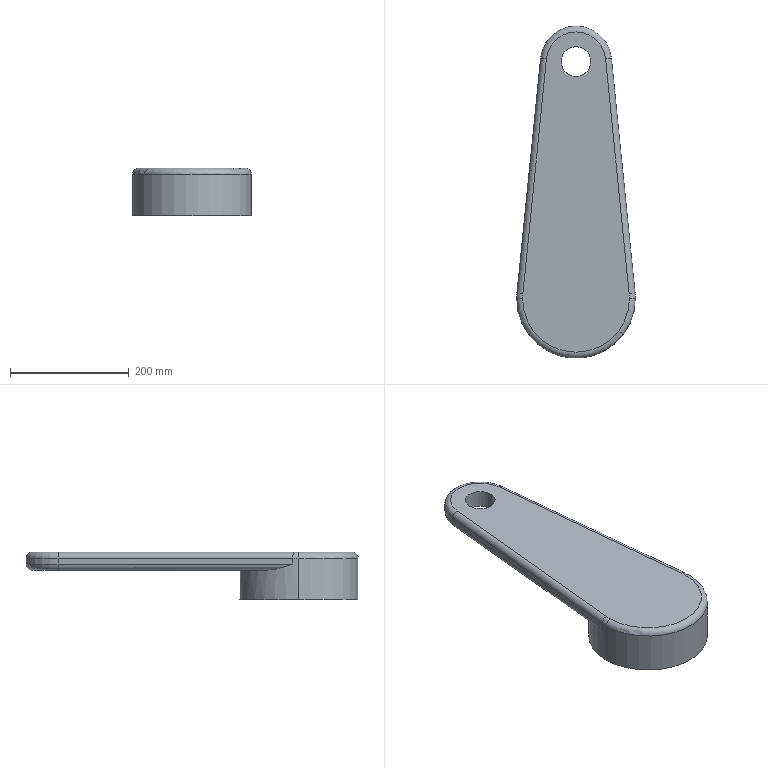Part | SolidWorks | features HoleWzd 2, Extrusion 1, Fillet 1, ICE 1 | 1 solid | 22 faces | box 200 x 560.023 x 80 mm | volume 3893750 mm3 | cylinder 11 | plane 6 | torus 5 | commonest cylinder face diameters 20 x4 50 x2 60 x2 200 x2 120.046 x1
STEP:
#1=CARTESIAN_POINT('',(90.,0.,30.));
#2=VERTEX_POINT('',#1);
#3=CARTESIAN_POINT('',(89.549,8.995,30.));
#4=VERTEX_POINT('',#3);
#5=CARTESIAN_POINT('',(0.,0.,30.));
#6=DIRECTION('',(0.,0.,1.));
#7=DIRECTION('',(-1.,0.,0.));
#8=AXIS2_PLACEMENT_3D('',#5,#6,#7);
#9=CIRCLE('',#8,90.);
#10=EDGE_CURVE('',#2,#4,#9,.T.);
#11=ORIENTED_EDGE('',*,*,#10,.F.);
#12=CARTESIAN_POINT('',(100.,0.,20.));
#13=VERTEX_POINT('',#12);
#14=CARTESIAN_POINT('',(90.,0.,20.));
#15=DIRECTION('',(0.,1.,0.));
#16=DIRECTION('',(-1.,0.,0.));
#17=AXIS2_PLACEMENT_3D('',#14,#15,#16);
#18=CIRCLE('',#17,10.);
#19=EDGE_CURVE('',#2,#13,#18,.T.);
#20=ORIENTED_EDGE('',*,*,#19,.T.);
#21=CARTESIAN_POINT('',(99.499,9.994,20.));
#22=VERTEX_POINT('',#21);
#23=CARTESIAN_POINT('',(0.,0.,20.));
#24=DIRECTION('',(0.,0.,-1.));
#25=DIRECTION('',(-1.,0.,0.));
#26=AXIS2_PLACEMENT_3D('',#23,#24,#25);
#27=CIRCLE('',#26,100.);
#28=EDGE_CURVE('',#22,#13,#27,.T.);
#29=ORIENTED_EDGE('',*,*,#28,.F.);
#30=CARTESIAN_POINT('',(89.549,8.995,20.));
#31=DIRECTION('',(0.09994,-0.995,0.));
#32=DIRECTION('',(0.995,0.09994,0.));
#33=AXIS2_PLACEMENT_3D('',#30,#31,#32);
#34=CIRCLE('',#33,10.);
#35=EDGE_CURVE('',#22,#4,#34,.T.);
#36=ORIENTED_EDGE('',*,*,#35,.T.);
#37=EDGE_LOOP('',(#11,#20,#29,#36));
#38=FACE_OUTER_BOUND('',#37,.T.);
#39=CARTESIAN_POINT('',(0.,0.,20.));
#40=DIRECTION('',(0.,0.,-1.));
#41=DIRECTION('',(-1.,0.,0.));
#42=AXIS2_PLACEMENT_3D('',#39,#40,#41);
#43=TOROIDAL_SURFACE('',#42,90.,10.);
#44=ADVANCED_FACE('',(#38),#43,.T.);
#45=ORIENTED_EDGE('',*,*,#19,.F.);
#46=CARTESIAN_POINT('',(-90.,0.,30.));
#47=VERTEX_POINT('',#46);
#48=CARTESIAN_POINT('',(0.,0.,30.));
#49=DIRECTION('',(0.,0.,1.));
#50=DIRECTION('',(-1.,0.,0.));
#51=AXIS2_PLACEMENT_3D('',#48,#49,#50);
#52=CIRCLE('',#51,90.);
#53=EDGE_CURVE('',#47,#2,#52,.T.);
#54=ORIENTED_EDGE('',*,*,#53,.F.);
#55=CARTESIAN_POINT('',(-100.,0.,20.));
#56=VERTEX_POINT('',#55);
#57=CARTESIAN_POINT('',(-90.,0.,20.));
#58=DIRECTION('',(0.,-1.,0.));
#59=DIRECTION('',(0.,0.,-1.));
#60=AXIS2_PLACEMENT_3D('',#57,#58,#59);
#61=CIRCLE('',#60,10.);
#62=EDGE_CURVE('',#47,#56,#61,.T.);
#63=ORIENTED_EDGE('',*,*,#62,.T.);
#64=CARTESIAN_POINT('',(0.,0.,20.));
#65=DIRECTION('',(0.,0.,-1.));
#66=DIRECTION('',(-1.,0.,0.));
#67=AXIS2_PLACEMENT_3D('',#64,#65,#66);
#68=CIRCLE('',#67,100.);
#69=EDGE_CURVE('',#13,#56,#68,.T.);
#70=ORIENTED_EDGE('',*,*,#69,.F.);
#71=EDGE_LOOP('',(#45,#54,#63,#70));
#72=FACE_OUTER_BOUND('',#71,.T.);
#73=CARTESIAN_POINT('',(0.,0.,20.));
#74=DIRECTION('',(0.,0.,-1.));
#75=DIRECTION('',(-1.,0.,0.));
#76=AXIS2_PLACEMENT_3D('',#73,#74,#75);
#77=TOROIDAL_SURFACE('',#76,90.,10.);
#78=ADVANCED_FACE('',(#72),#77,.T.);
#79=CARTESIAN_POINT('',(30.,0.,0.));
#80=VERTEX_POINT('',#79);
#81=CARTESIAN_POINT('',(-30.,0.,0.));
#82=VERTEX_POINT('',#81);
#83=CARTESIAN_POINT('',(0.,0.,0.));
#84=DIRECTION('',(0.,0.,-1.));
#85=DIRECTION('',(-1.,0.,0.));
#86=AXIS2_PLACEMENT_3D('',#83,#84,#85);
#87=CIRCLE('',#86,30.);
#88=EDGE_CURVE('',#80,#82,#87,.T.);
#89=ORIENTED_EDGE('',*,*,#88,.F.);
#90=CARTESIAN_POINT('',(30.,0.,-50.));
#91=VERTEX_POINT('',#90);
#92=CARTESIAN_POINT('',(30.,0.,-50.));
#93=DIRECTION('',(0.,0.,-1.));
#94=VECTOR('',#93,1000.);
#95=LINE('',#92,#94);
#96=EDGE_CURVE('',#80,#91,#95,.T.);
#97=ORIENTED_EDGE('',*,*,#96,.T.);
#98=CARTESIAN_POINT('',(-30.,0.,-50.));
#99=VERTEX_POINT('',#98);
#100=CARTESIAN_POINT('',(0.,0.,-50.));
#101=DIRECTION('',(0.,0.,-1.));
#102=DIRECTION('',(-1.,0.,0.));
#103=AXIS2_PLACEMENT_3D('',#100,#101,#102);
#104=CIRCLE('',#103,30.);
#105=EDGE_CURVE('',#91,#99,#104,.T.);
#106=ORIENTED_EDGE('',*,*,#105,.T.);
#107=CARTESIAN_POINT('',(-30.,0.,-50.));
#108=DIRECTION('',(0.,0.,-1.));
#109=VECTOR('',#108,1000.);
#110=LINE('',#107,#109);
#111=EDGE_CURVE('',#82,#99,#110,.T.);
#112=ORIENTED_EDGE('',*,*,#111,.F.);
#113=EDGE_LOOP('',(#89,#97,#106,#112));
#114=FACE_OUTER_BOUND('',#113,.T.);
#115=CARTESIAN_POINT('',(0.,0.,-50.));
#116=DIRECTION('',(0.,0.,-1.));
#117=DIRECTION('',(-1.,0.,0.));
#118=AXIS2_PLACEMENT_3D('',#115,#116,#117);
#119=CYLINDRICAL_SURFACE('',#118,30.);
#120=ADVANCED_FACE('',(#114),#119,.F.);
#121=CARTESIAN_POINT('',(25.,400.,30.));
#122=VERTEX_POINT('',#121);
#123=CARTESIAN_POINT('',(-25.,400.,30.));
#124=VERTEX_POINT('',#123);
#125=CARTESIAN_POINT('',(0.,400.,30.));
#126=DIRECTION('',(0.,0.,-1.));
#127=DIRECTION('',(-1.,0.,0.));
#128=AXIS2_PLACEMENT_3D('',#125,#126,#127);
#129=CIRCLE('',#128,25.);
#130=EDGE_CURVE('',#122,#124,#129,.T.);
#131=ORIENTED_EDGE('',*,*,#130,.F.);
#132=CARTESIAN_POINT('',(25.,400.,0.));
#133=VERTEX_POINT('',#132);
#134=CARTESIAN_POINT('',(25.,400.,0.));
#135=DIRECTION('',(0.,0.,-1.));
#136=VECTOR('',#135,1000.);
#137=LINE('',#134,#136);
#138=EDGE_CURVE('',#122,#133,#137,.T.);
#139=ORIENTED_EDGE('',*,*,#138,.T.);
#140=CARTESIAN_POINT('',(-25.,400.,0.));
#141=VERTEX_POINT('',#140);
#142=CARTESIAN_POINT('',(0.,400.,0.));
#143=DIRECTION('',(0.,0.,-1.));
#144=DIRECTION('',(-1.,0.,0.));
#145=AXIS2_PLACEMENT_3D('',#142,#143,#144);
#146=CIRCLE('',#145,25.);
#147=EDGE_CURVE('',#133,#141,#146,.T.);
#148=ORIENTED_EDGE('',*,*,#147,.T.);
#149=CARTESIAN_POINT('',(-25.,400.,0.));
#150=DIRECTION('',(0.,0.,-1.));
#151=VECTOR('',#150,1000.);
#152=LINE('',#149,#151);
#153=EDGE_CURVE('',#124,#141,#152,.T.);
#154=ORIENTED_EDGE('',*,*,#153,.F.);
#155=EDGE_LOOP('',(#131,#139,#148,#154));
#156=FACE_OUTER_BOUND('',#155,.T.);
#157=CARTESIAN_POINT('',(0.,400.,0.));
#158=DIRECTION('',(0.,0.,-1.));
#159=DIRECTION('',(-1.,0.,0.));
#160=AXIS2_PLACEMENT_3D('',#157,#158,#159);
#161=CYLINDRICAL_SURFACE('',#160,25.);
#162=ADVANCED_FACE('',(#156),#161,.F.);
#163=ORIENTED_EDGE('',*,*,#28,.T.);
#164=CARTESIAN_POINT('',(100.,0.,-50.));
#165=VERTEX_POINT('',#164);
#166=CARTESIAN_POINT('',(100.,0.,30.));
#167=DIRECTION('',(0.,0.,-1.));
#168=VECTOR('',#167,1000.);
#169=LINE('',#166,#168);
#170=EDGE_CURVE('',#13,#165,#169,.T.);
#171=ORIENTED_EDGE('',*,*,#170,.T.);
#172=CARTESIAN_POINT('',(-100.,0.,-50.));
#173=VERTEX_POINT('',#172);
#174=CARTESIAN_POINT('',(0.,0.,-50.));
#175=DIRECTION('',(0.,0.,-1.));
#176=DIRECTION('',(-1.,0.,0.));
#177=AXIS2_PLACEMENT_3D('',#174,#175,#176);
#178=CIRCLE('',#177,100.);
#179=EDGE_CURVE('',#173,#165,#178,.T.);
#180=ORIENTED_EDGE('',*,*,#179,.F.);
#181=CARTESIAN_POINT('',(-100.,0.,30.));
#182=DIRECTION('',(0.,0.,-1.));
#183=VECTOR('',#182,1000.);
#184=LINE('',#181,#183);
#185=EDGE_CURVE('',#56,#173,#184,.T.);
#186=ORIENTED_EDGE('',*,*,#185,.F.);
#187=CARTESIAN_POINT('',(-99.499,9.994,20.));
#188=VERTEX_POINT('',#187);
#189=CARTESIAN_POINT('',(0.,0.,20.));
#190=DIRECTION('',(0.,0.,-1.));
#191=DIRECTION('',(-1.,0.,0.));
#192=AXIS2_PLACEMENT_3D('',#189,#190,#191);
#193=CIRCLE('',#192,100.);
#194=EDGE_CURVE('',#56,#188,#193,.T.);
#195=ORIENTED_EDGE('',*,*,#194,.T.);
#196=CARTESIAN_POINT('',(-99.499,9.994,10.));
#197=VERTEX_POINT('',#196);
#198=CARTESIAN_POINT('',(-99.499,9.994,30.));
#199=DIRECTION('',(0.,0.,-1.));
#200=VECTOR('',#199,1000.);
#201=LINE('',#198,#200);
#202=EDGE_CURVE('',#188,#197,#201,.T.);
#203=ORIENTED_EDGE('',*,*,#202,.T.);
#204=CARTESIAN_POINT('',(-85.193,52.366,0.));
#205=VERTEX_POINT('',#204);
#206=CARTESIAN_POINT('',(-99.499,9.994,10.));
#207=CARTESIAN_POINT('',(-99.476,10.223,9.927));
#208=CARTESIAN_POINT('',(-99.452,10.454,9.854));
#209=CARTESIAN_POINT('',(-99.403,10.914,9.708));
#210=CARTESIAN_POINT('',(-99.326,11.603,9.489));
#211=CARTESIAN_POINT('',(-99.132,13.207,8.978));
#212=CARTESIAN_POINT('',(-98.936,14.576,8.544));
#213=CARTESIAN_POINT('',(-98.508,17.307,7.68));
#214=CARTESIAN_POINT('',(-98.173,19.118,7.111));
#215=CARTESIAN_POINT('',(-97.015,24.528,5.446));
#216=CARTESIAN_POINT('',(-96.043,28.102,4.387));
#217=CARTESIAN_POINT('',(-94.56,32.548,3.2));
#218=CARTESIAN_POINT('',(-94.249,33.436,2.97));
#219=CARTESIAN_POINT('',(-93.601,35.21,2.526));
#220=CARTESIAN_POINT('',(-93.263,36.097,2.312));
#221=CARTESIAN_POINT('',(-92.211,38.739,1.703));
#222=CARTESIAN_POINT('',(-91.46,40.482,1.339));
#223=CARTESIAN_POINT('',(-89.853,43.933,0.7212));
#224=CARTESIAN_POINT('',(-88.998,45.641,0.467));
#225=CARTESIAN_POINT('',(-87.179,49.026,0.1067));
#226=CARTESIAN_POINT('',(-86.215,50.702,0.));
#227=CARTESIAN_POINT('',(-85.193,52.366,0.));
#228=B_SPLINE_CURVE_WITH_KNOTS('',3,(#206,#207,#208,#209,#210,#211,#212,#213,#214,#215,#216,#217,#218,#219,#220,#221,#222,#223,#224,#225,#226,#227),.UNSPECIFIED.,.F.,.F.,(4,2,1,1,2,2,2,2,2,2,2,4),(-0.00006325,0.0006587,0.001381,0.002825,0.005713,0.01149,0.02304,0.02593,0.02882,0.03459,0.04037,0.04614),.UNSPECIFIED.);
#229=EDGE_CURVE('',#197,#205,#228,.T.);
#230=ORIENTED_EDGE('',*,*,#229,.T.);
#231=CARTESIAN_POINT('',(85.193,52.366,0.));
#232=VERTEX_POINT('',#231);
#233=CARTESIAN_POINT('',(0.,0.,0.));
#234=DIRECTION('',(0.,0.,-1.));
#235=DIRECTION('',(-1.,0.,0.));
#236=AXIS2_PLACEMENT_3D('',#233,#234,#235);
#237=CIRCLE('',#236,100.);
#238=EDGE_CURVE('',#205,#232,#237,.T.);
#239=ORIENTED_EDGE('',*,*,#238,.T.);
#240=CARTESIAN_POINT('',(99.499,9.994,10.));
#241=VERTEX_POINT('',#240);
#242=CARTESIAN_POINT('',(85.193,52.366,0.));
#243=CARTESIAN_POINT('',(86.215,50.702,0.));
#244=CARTESIAN_POINT('',(87.179,49.026,0.1067));
#245=CARTESIAN_POINT('',(88.998,45.641,0.4669));
#246=CARTESIAN_POINT('',(89.853,43.933,0.7212));
#247=CARTESIAN_POINT('',(91.46,40.482,1.339));
#248=CARTESIAN_POINT('',(92.211,38.739,1.703));
#249=CARTESIAN_POINT('',(93.263,36.097,2.312));
#250=CARTESIAN_POINT('',(93.601,35.21,2.526));
#251=CARTESIAN_POINT('',(94.249,33.436,2.97));
#252=CARTESIAN_POINT('',(94.56,32.548,3.2));
#253=CARTESIAN_POINT('',(96.043,28.102,4.387));
#254=CARTESIAN_POINT('',(97.015,24.528,5.446));
#255=CARTESIAN_POINT('',(98.173,19.118,7.111));
#256=CARTESIAN_POINT('',(98.508,17.307,7.68));
#257=CARTESIAN_POINT('',(98.936,14.576,8.544));
#258=CARTESIAN_POINT('',(99.066,13.663,8.833));
#259=CARTESIAN_POINT('',(99.243,12.29,9.27));
#260=CARTESIAN_POINT('',(99.326,11.603,9.489));
#261=CARTESIAN_POINT('',(99.403,10.914,9.708));
#262=CARTESIAN_POINT('',(99.452,10.454,9.854));
#263=CARTESIAN_POINT('',(99.476,10.223,9.927));
#264=CARTESIAN_POINT('',(99.499,9.994,10.));
#265=B_SPLINE_CURVE_WITH_KNOTS('',3,(#242,#243,#244,#245,#246,#247,#248,#249,#250,#251,#252,#253,#254,#255,#256,#257,#258,#259,#260,#261,#262,#263,#264),.UNSPECIFIED.,.F.,.F.,(4,2,2,2,2,2,2,2,2,1,2,4),(0.,0.005781,0.01156,0.01734,0.02023,0.02312,0.03469,0.04047,0.04336,0.0448,0.04553,0.04625),.UNSPECIFIED.);
#266=EDGE_CURVE('',#232,#241,#265,.T.);
#267=ORIENTED_EDGE('',*,*,#266,.T.);
#268=CARTESIAN_POINT('',(99.499,9.994,30.));
#269=DIRECTION('',(0.,0.,-1.));
#270=VECTOR('',#269,1000.);
#271=LINE('',#268,#270);
#272=EDGE_CURVE('',#22,#241,#271,.T.);
#273=ORIENTED_EDGE('',*,*,#272,.F.);
#274=EDGE_LOOP('',(#163,#171,#180,#186,#195,#203,#230,#239,#267,#273));
#275=FACE_OUTER_BOUND('',#274,.T.);
#276=CARTESIAN_POINT('',(0.,0.,30.));
#277=DIRECTION('',(0.,0.,-1.));
#278=DIRECTION('',(-1.,0.,0.));
#279=AXIS2_PLACEMENT_3D('',#276,#277,#278);
#280=CYLINDRICAL_SURFACE('',#279,100.);
#281=ADVANCED_FACE('',(#275),#280,.T.);
#282=CARTESIAN_POINT('',(-59.723,405.999,20.));
#283=VERTEX_POINT('',#282);
#284=CARTESIAN_POINT('',(-59.723,405.999,10.));
#285=VERTEX_POINT('',#284);
#286=CARTESIAN_POINT('',(-59.723,405.999,30.));
#287=DIRECTION('',(0.,0.,-1.));
#288=VECTOR('',#287,1000.);
#289=LINE('',#286,#288);
#290=EDGE_CURVE('',#283,#285,#289,.T.);
#291=ORIENTED_EDGE('',*,*,#290,.F.);
#292=CARTESIAN_POINT('',(59.723,405.999,20.));
#293=VERTEX_POINT('',#292);
#294=CARTESIAN_POINT('',(0.,400.,20.));
#295=DIRECTION('',(0.,0.,-1.));
#296=DIRECTION('',(-1.,0.,0.));
#297=AXIS2_PLACEMENT_3D('',#294,#295,#296);
#298=CIRCLE('',#297,60.023);
#299=EDGE_CURVE('',#283,#293,#298,.T.);
#300=ORIENTED_EDGE('',*,*,#299,.T.);
#301=CARTESIAN_POINT('',(59.723,405.999,10.));
#302=VERTEX_POINT('',#301);
#303=CARTESIAN_POINT('',(59.723,405.999,30.));
#304=DIRECTION('',(0.,0.,-1.));
#305=VECTOR('',#304,1000.);
#306=LINE('',#303,#305);
#307=EDGE_CURVE('',#293,#302,#306,.T.);
#308=ORIENTED_EDGE('',*,*,#307,.T.);
#309=CARTESIAN_POINT('',(0.,400.,10.));
#310=DIRECTION('',(0.,0.,1.));
#311=DIRECTION('',(-1.,0.,0.));
#312=AXIS2_PLACEMENT_3D('',#309,#310,#311);
#313=CIRCLE('',#312,60.023);
#314=EDGE_CURVE('',#302,#285,#313,.T.);
#315=ORIENTED_EDGE('',*,*,#314,.T.);
#316=EDGE_LOOP('',(#291,#300,#308,#315));
#317=FACE_OUTER_BOUND('',#316,.T.);
#318=CARTESIAN_POINT('',(0.,400.,30.));
#319=DIRECTION('',(0.,0.,-1.));
#320=DIRECTION('',(-1.,0.,0.));
#321=AXIS2_PLACEMENT_3D('',#318,#319,#320);
#322=CYLINDRICAL_SURFACE('',#321,60.023);
#323=ADVANCED_FACE('',(#317),#322,.T.);
#324=ORIENTED_EDGE('',*,*,#202,.F.);
#325=CARTESIAN_POINT('',(-59.723,405.999,20.));
#326=DIRECTION('',(0.09994,0.995,0.));
#327=VECTOR('',#326,1000.);
#328=LINE('',#325,#327);
#329=EDGE_CURVE('',#188,#283,#328,.T.);
#330=ORIENTED_EDGE('',*,*,#329,.T.);
#331=ORIENTED_EDGE('',*,*,#290,.T.);
#332=CARTESIAN_POINT('',(-99.499,9.994,10.));
#333=DIRECTION('',(-0.09994,-0.995,0.));
#334=VECTOR('',#333,1000.);
#335=LINE('',#332,#334);
#336=EDGE_CURVE('',#285,#197,#335,.T.);
#337=ORIENTED_EDGE('',*,*,#336,.T.);
#338=EDGE_LOOP('',(#324,#330,#331,#337));
#339=FACE_OUTER_BOUND('',#338,.T.);
#340=CARTESIAN_POINT('',(-99.499,9.994,30.));
#341=DIRECTION('',(-0.995,0.09994,0.));
#342=DIRECTION('',(-0.09994,-0.995,0.));
#343=AXIS2_PLACEMENT_3D('',#340,#341,#342);
#344=PLANE('',#343);
#345=ADVANCED_FACE('',(#339),#344,.T.);
#346=ORIENTED_EDGE('',*,*,#170,.F.);
#347=ORIENTED_EDGE('',*,*,#69,.T.);
#348=ORIENTED_EDGE('',*,*,#185,.T.);
#349=CARTESIAN_POINT('',(0.,0.,-50.));
#350=DIRECTION('',(0.,0.,-1.));
#351=DIRECTION('',(-1.,0.,0.));
#352=AXIS2_PLACEMENT_3D('',#349,#350,#351);
#353=CIRCLE('',#352,100.);
#354=EDGE_CURVE('',#165,#173,#353,.T.);
#355=ORIENTED_EDGE('',*,*,#354,.F.);
#356=EDGE_LOOP('',(#346,#347,#348,#355));
#357=FACE_OUTER_BOUND('',#356,.T.);
#358=CARTESIAN_POINT('',(0.,0.,30.));
#359=DIRECTION('',(0.,0.,-1.));
#360=DIRECTION('',(-1.,0.,0.));
#361=AXIS2_PLACEMENT_3D('',#358,#359,#360);
#362=CYLINDRICAL_SURFACE('',#361,100.);
#363=ADVANCED_FACE('',(#357),#362,.T.);
#364=ORIENTED_EDGE('',*,*,#307,.F.);
#365=CARTESIAN_POINT('',(99.499,9.994,20.));
#366=DIRECTION('',(0.09994,-0.995,0.));
#367=VECTOR('',#366,1000.);
#368=LINE('',#365,#367);
#369=EDGE_CURVE('',#293,#22,#368,.T.);
#370=ORIENTED_EDGE('',*,*,#369,.T.);
#371=ORIENTED_EDGE('',*,*,#272,.T.);
#372=CARTESIAN_POINT('',(59.723,405.999,10.));
#373=DIRECTION('',(-0.09994,0.995,0.));
#374=VECTOR('',#373,1000.);
#375=LINE('',#372,#374);
#376=EDGE_CURVE('',#241,#302,#375,.T.);
#377=ORIENTED_EDGE('',*,*,#376,.T.);
#378=EDGE_LOOP('',(#364,#370,#371,#377));
#379=FACE_OUTER_BOUND('',#378,.T.);
#380=CARTESIAN_POINT('',(59.723,405.999,30.));
#381=DIRECTION('',(0.995,0.09994,0.));
#382=DIRECTION('',(-0.09994,0.995,0.));
#383=AXIS2_PLACEMENT_3D('',#380,#381,#382);
#384=PLANE('',#383);
#385=ADVANCED_FACE('',(#379),#384,.T.);
#386=CARTESIAN_POINT('',(-49.773,404.999,30.));
#387=VERTEX_POINT('',#386);
#388=CARTESIAN_POINT('',(-89.549,8.995,30.));
#389=VERTEX_POINT('',#388);
#390=CARTESIAN_POINT('',(-89.549,8.995,30.));
#391=DIRECTION('',(-0.09994,-0.995,0.));
#392=VECTOR('',#391,1000.);
#393=LINE('',#390,#392);
#394=EDGE_CURVE('',#387,#389,#393,.T.);
#395=ORIENTED_EDGE('',*,*,#394,.T.);
#396=CARTESIAN_POINT('',(0.,0.,30.));
#397=DIRECTION('',(0.,0.,1.));
#398=DIRECTION('',(-1.,0.,0.));
#399=AXIS2_PLACEMENT_3D('',#396,#397,#398);
#400=CIRCLE('',#399,90.);
#401=EDGE_CURVE('',#389,#47,#400,.T.);
#402=ORIENTED_EDGE('',*,*,#401,.T.);
#403=ORIENTED_EDGE('',*,*,#53,.T.);
#404=ORIENTED_EDGE('',*,*,#10,.T.);
#405=CARTESIAN_POINT('',(49.773,404.999,30.));
#406=VERTEX_POINT('',#405);
#407=CARTESIAN_POINT('',(49.773,404.999,30.));
#408=DIRECTION('',(-0.09994,0.995,0.));
#409=VECTOR('',#408,1000.);
#410=LINE('',#407,#409);
#411=EDGE_CURVE('',#4,#406,#410,.T.);
#412=ORIENTED_EDGE('',*,*,#411,.T.);
#413=CARTESIAN_POINT('',(0.,400.,30.));
#414=DIRECTION('',(0.,0.,1.));
#415=DIRECTION('',(-1.,0.,0.));
#416=AXIS2_PLACEMENT_3D('',#413,#414,#415);
#417=CIRCLE('',#416,50.023);
#418=EDGE_CURVE('',#406,#387,#417,.T.);
#419=ORIENTED_EDGE('',*,*,#418,.T.);
#420=EDGE_LOOP('',(#395,#402,#403,#404,#412,#419));
#421=FACE_OUTER_BOUND('',#420,.T.);
#422=CARTESIAN_POINT('',(0.,400.,30.));
#423=DIRECTION('',(0.,0.,-1.));
#424=DIRECTION('',(-1.,0.,0.));
#425=AXIS2_PLACEMENT_3D('',#422,#423,#424);
#426=CIRCLE('',#425,25.);
#427=EDGE_CURVE('',#124,#122,#426,.T.);
#428=ORIENTED_EDGE('',*,*,#427,.T.);
#429=ORIENTED_EDGE('',*,*,#130,.T.);
#430=EDGE_LOOP('',(#428,#429));
#431=FACE_BOUND('',#430,.T.);
#432=CARTESIAN_POINT('',(0.,400.,30.));
#433=DIRECTION('',(0.,0.,-1.));
#434=DIRECTION('',(-1.,0.,0.));
#435=AXIS2_PLACEMENT_3D('',#432,#433,#434);
#436=PLANE('',#435);
#437=ADVANCED_FACE('',(#421,#431),#436,.F.);
#438=ORIENTED_EDGE('',*,*,#238,.F.);
#439=CARTESIAN_POINT('',(-49.773,404.999,0.));
#440=VERTEX_POINT('',#439);
#441=CARTESIAN_POINT('',(-49.773,404.999,0.));
#442=DIRECTION('',(0.09994,0.995,0.));
#443=VECTOR('',#442,1000.);
#444=LINE('',#441,#443);
#445=EDGE_CURVE('',#205,#440,#444,.T.);
#446=ORIENTED_EDGE('',*,*,#445,.T.);
#447=CARTESIAN_POINT('',(49.773,404.999,0.));
#448=VERTEX_POINT('',#447);
#449=CARTESIAN_POINT('',(0.,400.,0.));
#450=DIRECTION('',(0.,0.,-1.));
#451=DIRECTION('',(-1.,0.,0.));
#452=AXIS2_PLACEMENT_3D('',#449,#450,#451);
#453=CIRCLE('',#452,50.023);
#454=EDGE_CURVE('',#440,#448,#453,.T.);
#455=ORIENTED_EDGE('',*,*,#454,.T.);
#456=CARTESIAN_POINT('',(49.773,404.999,0.));
#457=DIRECTION('',(0.09994,-0.995,0.));
#458=VECTOR('',#457,1000.);
#459=LINE('',#456,#458);
#460=EDGE_CURVE('',#448,#232,#459,.T.);
#461=ORIENTED_EDGE('',*,*,#460,.T.);
#462=EDGE_LOOP('',(#438,#446,#455,#461));
#463=FACE_OUTER_BOUND('',#462,.T.);
#464=CARTESIAN_POINT('',(0.,400.,0.));
#465=DIRECTION('',(0.,0.,-1.));
#466=DIRECTION('',(-1.,0.,0.));
#467=AXIS2_PLACEMENT_3D('',#464,#465,#466);
#468=CIRCLE('',#467,25.);
#469=EDGE_CURVE('',#141,#133,#468,.T.);
#470=ORIENTED_EDGE('',*,*,#469,.F.);
#471=ORIENTED_EDGE('',*,*,#147,.F.);
#472=EDGE_LOOP('',(#470,#471));
#473=FACE_BOUND('',#472,.T.);
#474=CARTESIAN_POINT('',(0.,400.,0.));
#475=DIRECTION('',(0.,0.,-1.));
#476=DIRECTION('',(-1.,0.,0.));
#477=AXIS2_PLACEMENT_3D('',#474,#475,#476);
#478=PLANE('',#477);
#479=ADVANCED_FACE('',(#463,#473),#478,.T.);
#480=CARTESIAN_POINT('',(0.,0.,-50.));
#481=DIRECTION('',(0.,0.,-1.));
#482=DIRECTION('',(-1.,0.,0.));
#483=AXIS2_PLACEMENT_3D('',#480,#481,#482);
#484=CIRCLE('',#483,30.);
#485=EDGE_CURVE('',#99,#91,#484,.T.);
#486=ORIENTED_EDGE('',*,*,#485,.F.);
#487=ORIENTED_EDGE('',*,*,#105,.F.);
#488=EDGE_LOOP('',(#486,#487));
#489=FACE_BOUND('',#488,.T.);
#490=ORIENTED_EDGE('',*,*,#179,.T.);
#491=ORIENTED_EDGE('',*,*,#354,.T.);
#492=EDGE_LOOP('',(#490,#491));
#493=FACE_OUTER_BOUND('',#492,.T.);
#494=CARTESIAN_POINT('',(0.,0.,-50.));
#495=DIRECTION('',(0.,0.,-1.));
#496=DIRECTION('',(-1.,0.,0.));
#497=AXIS2_PLACEMENT_3D('',#494,#495,#496);
#498=PLANE('',#497);
#499=ADVANCED_FACE('',(#489,#493),#498,.T.);
#500=ORIENTED_EDGE('',*,*,#138,.F.);
#501=ORIENTED_EDGE('',*,*,#427,.F.);
#502=ORIENTED_EDGE('',*,*,#153,.T.);
#503=ORIENTED_EDGE('',*,*,#469,.T.);
#504=EDGE_LOOP('',(#500,#501,#502,#503));
#505=FACE_OUTER_BOUND('',#504,.T.);
#506=CARTESIAN_POINT('',(0.,400.,0.));
#507=DIRECTION('',(0.,0.,-1.));
#508=DIRECTION('',(-1.,0.,0.));
#509=AXIS2_PLACEMENT_3D('',#506,#507,#508);
#510=CYLINDRICAL_SURFACE('',#509,25.);
#511=ADVANCED_FACE('',(#505),#510,.F.);
#512=CARTESIAN_POINT('',(0.,0.,0.));
#513=DIRECTION('',(0.,0.,-1.));
#514=DIRECTION('',(-1.,0.,0.));
#515=AXIS2_PLACEMENT_3D('',#512,#513,#514);
#516=CIRCLE('',#515,30.);
#517=EDGE_CURVE('',#82,#80,#516,.T.);
#518=ORIENTED_EDGE('',*,*,#517,.T.);
#519=ORIENTED_EDGE('',*,*,#88,.T.);
#520=EDGE_LOOP('',(#518,#519));
#521=FACE_OUTER_BOUND('',#520,.T.);
#522=CARTESIAN_POINT('',(0.,0.,0.));
#523=DIRECTION('',(0.,0.,1.));
#524=DIRECTION('',(1.,0.,0.));
#525=AXIS2_PLACEMENT_3D('',#522,#523,#524);
#526=PLANE('',#525);
#527=ADVANCED_FACE('',(#521),#526,.F.);
#528=ORIENTED_EDGE('',*,*,#96,.F.);
#529=ORIENTED_EDGE('',*,*,#517,.F.);
#530=ORIENTED_EDGE('',*,*,#111,.T.);
#531=ORIENTED_EDGE('',*,*,#485,.T.);
#532=EDGE_LOOP('',(#528,#529,#530,#531));
#533=FACE_OUTER_BOUND('',#532,.T.);
#534=CARTESIAN_POINT('',(0.,0.,-50.));
#535=DIRECTION('',(0.,0.,-1.));
#536=DIRECTION('',(-1.,0.,0.));
#537=AXIS2_PLACEMENT_3D('',#534,#535,#536);
#538=CYLINDRICAL_SURFACE('',#537,30.);
#539=ADVANCED_FACE('',(#533),#538,.F.);
#540=CARTESIAN_POINT('',(-49.773,404.999,20.));
#541=DIRECTION('',(-0.09994,-0.995,0.));
#542=DIRECTION('',(0.995,-0.09994,0.));
#543=AXIS2_PLACEMENT_3D('',#540,#541,#542);
#544=CIRCLE('',#543,10.);
#545=EDGE_CURVE('',#387,#283,#544,.T.);
#546=ORIENTED_EDGE('',*,*,#545,.F.);
#547=ORIENTED_EDGE('',*,*,#418,.F.);
#548=CARTESIAN_POINT('',(49.773,404.999,20.));
#549=DIRECTION('',(0.09994,-0.995,0.));
#550=DIRECTION('',(0.995,0.09994,0.));
#551=AXIS2_PLACEMENT_3D('',#548,#549,#550);
#552=CIRCLE('',#551,10.);
#553=EDGE_CURVE('',#293,#406,#552,.T.);
#554=ORIENTED_EDGE('',*,*,#553,.F.);
#555=ORIENTED_EDGE('',*,*,#299,.F.);
#556=EDGE_LOOP('',(#546,#547,#554,#555));
#557=FACE_OUTER_BOUND('',#556,.T.);
#558=CARTESIAN_POINT('',(0.,400.,20.));
#559=DIRECTION('',(0.,0.,-1.));
#560=DIRECTION('',(-1.,0.,0.));
#561=AXIS2_PLACEMENT_3D('',#558,#559,#560);
#562=TOROIDAL_SURFACE('',#561,50.023,10.);
#563=ADVANCED_FACE('',(#557),#562,.T.);
#564=ORIENTED_EDGE('',*,*,#553,.T.);
#565=ORIENTED_EDGE('',*,*,#411,.F.);
#566=ORIENTED_EDGE('',*,*,#35,.F.);
#567=ORIENTED_EDGE('',*,*,#369,.F.);
#568=EDGE_LOOP('',(#564,#565,#566,#567));
#569=FACE_OUTER_BOUND('',#568,.T.);
#570=CARTESIAN_POINT('',(49.773,404.999,20.));
#571=DIRECTION('',(-0.09994,0.995,0.));
#572=DIRECTION('',(-0.995,-0.09994,0.));
#573=AXIS2_PLACEMENT_3D('',#570,#571,#572);
#574=CYLINDRICAL_SURFACE('',#573,10.);
#575=ADVANCED_FACE('',(#569),#574,.T.);
#576=ORIENTED_EDGE('',*,*,#545,.T.);
#577=ORIENTED_EDGE('',*,*,#329,.F.);
#578=CARTESIAN_POINT('',(-89.549,8.995,20.));
#579=DIRECTION('',(-0.09994,-0.995,0.));
#580=DIRECTION('',(0.995,-0.09994,0.));
#581=AXIS2_PLACEMENT_3D('',#578,#579,#580);
#582=CIRCLE('',#581,10.);
#583=EDGE_CURVE('',#389,#188,#582,.T.);
#584=ORIENTED_EDGE('',*,*,#583,.F.);
#585=ORIENTED_EDGE('',*,*,#394,.F.);
#586=EDGE_LOOP('',(#576,#577,#584,#585));
#587=FACE_OUTER_BOUND('',#586,.T.);
#588=CARTESIAN_POINT('',(-89.549,8.995,20.));
#589=DIRECTION('',(-0.09994,-0.995,0.));
#590=DIRECTION('',(0.995,-0.09994,0.));
#591=AXIS2_PLACEMENT_3D('',#588,#589,#590);
#592=CYLINDRICAL_SURFACE('',#591,10.);
#593=ADVANCED_FACE('',(#587),#592,.T.);
#594=ORIENTED_EDGE('',*,*,#62,.F.);
#595=ORIENTED_EDGE('',*,*,#401,.F.);
#596=ORIENTED_EDGE('',*,*,#583,.T.);
#597=ORIENTED_EDGE('',*,*,#194,.F.);
#598=EDGE_LOOP('',(#594,#595,#596,#597));
#599=FACE_OUTER_BOUND('',#598,.T.);
#600=CARTESIAN_POINT('',(0.,0.,20.));
#601=DIRECTION('',(0.,0.,-1.));
#602=DIRECTION('',(-1.,0.,0.));
#603=AXIS2_PLACEMENT_3D('',#600,#601,#602);
#604=TOROIDAL_SURFACE('',#603,90.,10.);
#605=ADVANCED_FACE('',(#599),#604,.T.);
#606=ORIENTED_EDGE('',*,*,#266,.F.);
#607=ORIENTED_EDGE('',*,*,#460,.F.);
#608=CARTESIAN_POINT('',(49.773,404.999,10.));
#609=DIRECTION('',(-0.09994,0.995,0.));
#610=DIRECTION('',(-0.995,-0.09994,0.));
#611=AXIS2_PLACEMENT_3D('',#608,#609,#610);
#612=CIRCLE('',#611,10.);
#613=EDGE_CURVE('',#302,#448,#612,.T.);
#614=ORIENTED_EDGE('',*,*,#613,.F.);
#615=ORIENTED_EDGE('',*,*,#376,.F.);
#616=EDGE_LOOP('',(#606,#607,#614,#615));
#617=FACE_OUTER_BOUND('',#616,.T.);
#618=CARTESIAN_POINT('',(49.773,404.999,10.));
#619=DIRECTION('',(0.09994,-0.995,0.));
#620=DIRECTION('',(0.995,0.09994,0.));
#621=AXIS2_PLACEMENT_3D('',#618,#619,#620);
#622=CYLINDRICAL_SURFACE('',#621,10.);
#623=ADVANCED_FACE('',(#617),#622,.T.);
#624=ORIENTED_EDGE('',*,*,#613,.T.);
#625=ORIENTED_EDGE('',*,*,#454,.F.);
#626=CARTESIAN_POINT('',(-49.773,404.999,10.));
#627=DIRECTION('',(-0.09994,-0.995,0.));
#628=DIRECTION('',(0.995,-0.09994,0.));
#629=AXIS2_PLACEMENT_3D('',#626,#627,#628);
#630=CIRCLE('',#629,10.);
#631=EDGE_CURVE('',#285,#440,#630,.T.);
#632=ORIENTED_EDGE('',*,*,#631,.F.);
#633=ORIENTED_EDGE('',*,*,#314,.F.);
#634=EDGE_LOOP('',(#624,#625,#632,#633));
#635=FACE_OUTER_BOUND('',#634,.T.);
#636=CARTESIAN_POINT('',(0.,400.,10.));
#637=DIRECTION('',(0.,0.,-1.));
#638=DIRECTION('',(-1.,0.,0.));
#639=AXIS2_PLACEMENT_3D('',#636,#637,#638);
#640=TOROIDAL_SURFACE('',#639,50.023,10.);
#641=ADVANCED_FACE('',(#635),#640,.T.);
#642=ORIENTED_EDGE('',*,*,#229,.F.);
#643=ORIENTED_EDGE('',*,*,#336,.F.);
#644=ORIENTED_EDGE('',*,*,#631,.T.);
#645=ORIENTED_EDGE('',*,*,#445,.F.);
#646=EDGE_LOOP('',(#642,#643,#644,#645));
#647=FACE_OUTER_BOUND('',#646,.T.);
#648=CARTESIAN_POINT('',(-49.773,404.999,10.));
#649=DIRECTION('',(0.09994,0.995,0.));
#650=DIRECTION('',(-0.995,0.09994,0.));
#651=AXIS2_PLACEMENT_3D('',#648,#649,#650);
#652=CYLINDRICAL_SURFACE('',#651,10.);
#653=ADVANCED_FACE('',(#647),#652,.T.);
#654=CLOSED_SHELL('',(#44,#78,#120,#162,#281,#323,#345,#363,#385,#437,#479,#499,#511,#527,#539,#563,#575,#593,#605,#623,#641,#653));
#655=MANIFOLD_SOLID_BREP('',#654);
#656=CARTESIAN_POINT('',(0.,0.,0.));
#657=DIRECTION('',(0.,0.,1.));
#658=DIRECTION('',(1.,0.,0.));
#659=AXIS2_PLACEMENT_3D('',#656,#657,#658);
#660=(LENGTH_UNIT()NAMED_UNIT(*)SI_UNIT(.MILLI.,.METRE.));
#661=UNCERTAINTY_MEASURE_WITH_UNIT(LENGTH_MEASURE(0.00001),#660,'','');
#662=(NAMED_UNIT(*)PLANE_ANGLE_UNIT()SI_UNIT($,.RADIAN.));
#663=(NAMED_UNIT(*)SI_UNIT($,.STERADIAN.)SOLID_ANGLE_UNIT());
#664=(GEOMETRIC_REPRESENTATION_CONTEXT(3)GLOBAL_UNCERTAINTY_ASSIGNED_CONTEXT((#661))GLOBAL_UNIT_ASSIGNED_CONTEXT((#660,#662,#663))REPRESENTATION_CONTEXT('',''));
#665=ADVANCED_BREP_SHAPE_REPRESENTATION('',(#655,#659),#664);